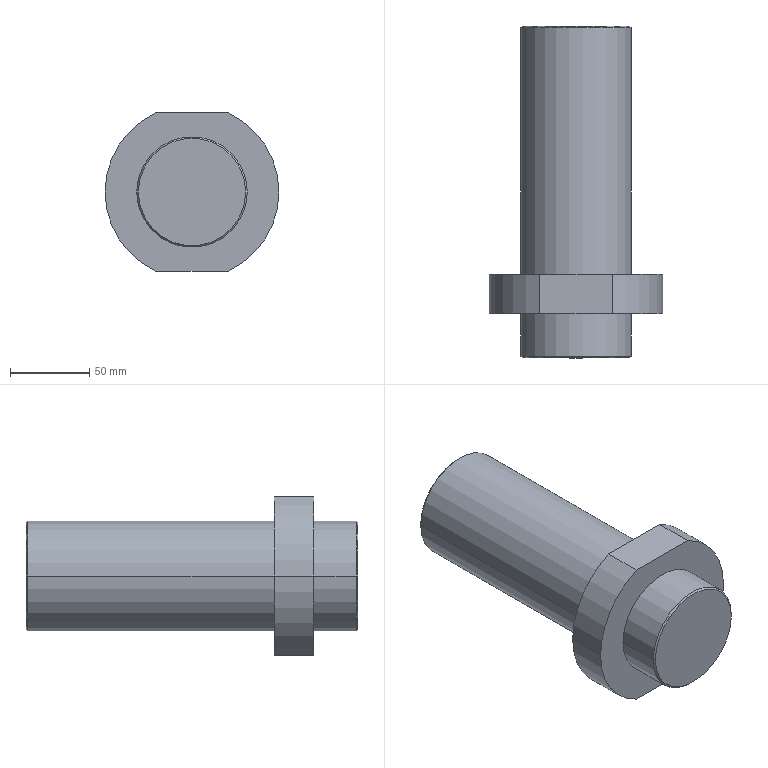Part | SolidWorks | features ICE 1, Revolution 1 | 1 solid | 17 faces | box 110 x 210 x 100 mm | volume 941619 mm3 | cylinder 7 | plane 6 | cone 4 | commonest cylinder face diameters 70 x4 110 x3
STEP:
#1=CARTESIAN_POINT('',(-34.,210.,0.));
#2=VERTEX_POINT('',#1);
#3=CARTESIAN_POINT('',(34.,210.,0.));
#4=VERTEX_POINT('',#3);
#5=CARTESIAN_POINT('',(0.,210.,0.));
#6=DIRECTION('',(0.,1.,0.));
#7=DIRECTION('',(-1.,0.,0.));
#8=AXIS2_PLACEMENT_3D('',#5,#6,#7);
#9=CIRCLE('',#8,34.);
#10=EDGE_CURVE('',#2,#4,#9,.T.);
#11=ORIENTED_EDGE('',*,*,#10,.F.);
#12=CARTESIAN_POINT('',(-35.,209.,0.));
#13=VERTEX_POINT('',#12);
#14=CARTESIAN_POINT('',(-34.,210.,0.));
#15=DIRECTION('',(-0.7071,-0.7071,0.));
#16=VECTOR('',#15,1000.);
#17=LINE('',#14,#16);
#18=EDGE_CURVE('',#2,#13,#17,.T.);
#19=ORIENTED_EDGE('',*,*,#18,.T.);
#20=CARTESIAN_POINT('',(35.,209.,0.));
#21=VERTEX_POINT('',#20);
#22=CARTESIAN_POINT('',(0.,209.,0.));
#23=DIRECTION('',(0.,1.,0.));
#24=DIRECTION('',(-1.,0.,0.));
#25=AXIS2_PLACEMENT_3D('',#22,#23,#24);
#26=CIRCLE('',#25,35.);
#27=EDGE_CURVE('',#13,#21,#26,.T.);
#28=ORIENTED_EDGE('',*,*,#27,.T.);
#29=CARTESIAN_POINT('',(34.,210.,0.));
#30=DIRECTION('',(0.7071,-0.7071,0.));
#31=VECTOR('',#30,1000.);
#32=LINE('',#29,#31);
#33=EDGE_CURVE('',#4,#21,#32,.T.);
#34=ORIENTED_EDGE('',*,*,#33,.F.);
#35=EDGE_LOOP('',(#11,#19,#28,#34));
#36=FACE_OUTER_BOUND('',#35,.T.);
#37=CARTESIAN_POINT('',(0.,210.,0.));
#38=DIRECTION('',(0.,-1.,0.));
#39=DIRECTION('',(1.,0.,0.));
#40=AXIS2_PLACEMENT_3D('',#37,#38,#39);
#41=CONICAL_SURFACE('',#40,34.,0.7854);
#42=ADVANCED_FACE('',(#36),#41,.T.);
#43=CARTESIAN_POINT('',(-35.,53.,0.));
#44=VERTEX_POINT('',#43);
#45=CARTESIAN_POINT('',(35.,53.,0.));
#46=VERTEX_POINT('',#45);
#47=CARTESIAN_POINT('',(0.,53.,0.));
#48=DIRECTION('',(0.,1.,0.));
#49=DIRECTION('',(-1.,0.,0.));
#50=AXIS2_PLACEMENT_3D('',#47,#48,#49);
#51=CIRCLE('',#50,35.);
#52=EDGE_CURVE('',#44,#46,#51,.T.);
#53=ORIENTED_EDGE('',*,*,#52,.T.);
#54=CARTESIAN_POINT('',(35.,210.,0.));
#55=DIRECTION('',(0.,1.,0.));
#56=VECTOR('',#55,1000.);
#57=LINE('',#54,#56);
#58=EDGE_CURVE('',#46,#21,#57,.T.);
#59=ORIENTED_EDGE('',*,*,#58,.T.);
#60=ORIENTED_EDGE('',*,*,#27,.F.);
#61=CARTESIAN_POINT('',(-35.,210.,0.));
#62=DIRECTION('',(0.,1.,0.));
#63=VECTOR('',#62,1000.);
#64=LINE('',#61,#63);
#65=EDGE_CURVE('',#44,#13,#64,.T.);
#66=ORIENTED_EDGE('',*,*,#65,.F.);
#67=EDGE_LOOP('',(#53,#59,#60,#66));
#68=FACE_OUTER_BOUND('',#67,.T.);
#69=CARTESIAN_POINT('',(0.,210.,0.));
#70=DIRECTION('',(0.,1.,0.));
#71=DIRECTION('',(-1.,0.,0.));
#72=AXIS2_PLACEMENT_3D('',#69,#70,#71);
#73=CYLINDRICAL_SURFACE('',#72,35.);
#74=ADVANCED_FACE('',(#68),#73,.T.);
#75=CARTESIAN_POINT('',(-35.,1.,0.));
#76=VERTEX_POINT('',#75);
#77=CARTESIAN_POINT('',(35.,1.,0.));
#78=VERTEX_POINT('',#77);
#79=CARTESIAN_POINT('',(0.,1.,0.));
#80=DIRECTION('',(0.,1.,0.));
#81=DIRECTION('',(-1.,0.,0.));
#82=AXIS2_PLACEMENT_3D('',#79,#80,#81);
#83=CIRCLE('',#82,35.);
#84=EDGE_CURVE('',#76,#78,#83,.T.);
#85=ORIENTED_EDGE('',*,*,#84,.T.);
#86=CARTESIAN_POINT('',(35.,28.,0.));
#87=VERTEX_POINT('',#86);
#88=CARTESIAN_POINT('',(35.,210.,0.));
#89=DIRECTION('',(0.,1.,0.));
#90=VECTOR('',#89,1000.);
#91=LINE('',#88,#90);
#92=EDGE_CURVE('',#78,#87,#91,.T.);
#93=ORIENTED_EDGE('',*,*,#92,.T.);
#94=CARTESIAN_POINT('',(-35.,28.,0.));
#95=VERTEX_POINT('',#94);
#96=CARTESIAN_POINT('',(0.,28.,0.));
#97=DIRECTION('',(0.,1.,0.));
#98=DIRECTION('',(-1.,0.,0.));
#99=AXIS2_PLACEMENT_3D('',#96,#97,#98);
#100=CIRCLE('',#99,35.);
#101=EDGE_CURVE('',#95,#87,#100,.T.);
#102=ORIENTED_EDGE('',*,*,#101,.F.);
#103=CARTESIAN_POINT('',(-35.,210.,0.));
#104=DIRECTION('',(0.,1.,0.));
#105=VECTOR('',#104,1000.);
#106=LINE('',#103,#105);
#107=EDGE_CURVE('',#76,#95,#106,.T.);
#108=ORIENTED_EDGE('',*,*,#107,.F.);
#109=EDGE_LOOP('',(#85,#93,#102,#108));
#110=FACE_OUTER_BOUND('',#109,.T.);
#111=CARTESIAN_POINT('',(0.,210.,0.));
#112=DIRECTION('',(0.,1.,0.));
#113=DIRECTION('',(-1.,0.,0.));
#114=AXIS2_PLACEMENT_3D('',#111,#112,#113);
#115=CYLINDRICAL_SURFACE('',#114,35.);
#116=ADVANCED_FACE('',(#110),#115,.T.);
#117=CARTESIAN_POINT('',(-34.,0.,0.));
#118=VERTEX_POINT('',#117);
#119=CARTESIAN_POINT('',(34.,0.,0.));
#120=VERTEX_POINT('',#119);
#121=CARTESIAN_POINT('',(0.,0.,0.));
#122=DIRECTION('',(0.,1.,0.));
#123=DIRECTION('',(-1.,0.,0.));
#124=AXIS2_PLACEMENT_3D('',#121,#122,#123);
#125=CIRCLE('',#124,34.);
#126=EDGE_CURVE('',#118,#120,#125,.T.);
#127=ORIENTED_EDGE('',*,*,#126,.T.);
#128=CARTESIAN_POINT('',(35.,1.,0.));
#129=DIRECTION('',(0.7071,0.7071,0.));
#130=VECTOR('',#129,1000.);
#131=LINE('',#128,#130);
#132=EDGE_CURVE('',#120,#78,#131,.T.);
#133=ORIENTED_EDGE('',*,*,#132,.T.);
#134=ORIENTED_EDGE('',*,*,#84,.F.);
#135=CARTESIAN_POINT('',(-35.,1.,0.));
#136=DIRECTION('',(-0.7071,0.7071,0.));
#137=VECTOR('',#136,1000.);
#138=LINE('',#135,#137);
#139=EDGE_CURVE('',#118,#76,#138,.T.);
#140=ORIENTED_EDGE('',*,*,#139,.F.);
#141=EDGE_LOOP('',(#127,#133,#134,#140));
#142=FACE_OUTER_BOUND('',#141,.T.);
#143=CARTESIAN_POINT('',(0.,1.,0.));
#144=DIRECTION('',(0.,1.,0.));
#145=DIRECTION('',(-1.,0.,0.));
#146=AXIS2_PLACEMENT_3D('',#143,#144,#145);
#147=CONICAL_SURFACE('',#146,35.,0.7854);
#148=ADVANCED_FACE('',(#142),#147,.T.);
#149=CARTESIAN_POINT('',(-22.913,28.,-50.));
#150=VERTEX_POINT('',#149);
#151=CARTESIAN_POINT('',(-55.,28.,0.));
#152=VERTEX_POINT('',#151);
#153=CARTESIAN_POINT('',(0.,28.,0.));
#154=DIRECTION('',(0.,1.,0.));
#155=DIRECTION('',(-1.,0.,0.));
#156=AXIS2_PLACEMENT_3D('',#153,#154,#155);
#157=CIRCLE('',#156,55.);
#158=EDGE_CURVE('',#150,#152,#157,.T.);
#159=ORIENTED_EDGE('',*,*,#158,.T.);
#160=CARTESIAN_POINT('',(-55.,53.,0.));
#161=VERTEX_POINT('',#160);
#162=CARTESIAN_POINT('',(-55.,210.,0.));
#163=DIRECTION('',(0.,1.,0.));
#164=VECTOR('',#163,1000.);
#165=LINE('',#162,#164);
#166=EDGE_CURVE('',#152,#161,#165,.T.);
#167=ORIENTED_EDGE('',*,*,#166,.T.);
#168=CARTESIAN_POINT('',(-22.913,53.,-50.));
#169=VERTEX_POINT('',#168);
#170=CARTESIAN_POINT('',(0.,53.,0.));
#171=DIRECTION('',(0.,1.,0.));
#172=DIRECTION('',(-1.,0.,0.));
#173=AXIS2_PLACEMENT_3D('',#170,#171,#172);
#174=CIRCLE('',#173,55.);
#175=EDGE_CURVE('',#169,#161,#174,.T.);
#176=ORIENTED_EDGE('',*,*,#175,.F.);
#177=CARTESIAN_POINT('',(-22.913,0.,-50.));
#178=DIRECTION('',(0.,1.,0.));
#179=VECTOR('',#178,1000.);
#180=LINE('',#177,#179);
#181=EDGE_CURVE('',#150,#169,#180,.T.);
#182=ORIENTED_EDGE('',*,*,#181,.F.);
#183=EDGE_LOOP('',(#159,#167,#176,#182));
#184=FACE_OUTER_BOUND('',#183,.T.);
#185=CARTESIAN_POINT('',(0.,210.,0.));
#186=DIRECTION('',(0.,1.,0.));
#187=DIRECTION('',(-1.,0.,0.));
#188=AXIS2_PLACEMENT_3D('',#185,#186,#187);
#189=CYLINDRICAL_SURFACE('',#188,55.);
#190=ADVANCED_FACE('',(#184),#189,.T.);
#191=ORIENTED_EDGE('',*,*,#166,.F.);
#192=CARTESIAN_POINT('',(-22.913,28.,50.));
#193=VERTEX_POINT('',#192);
#194=CARTESIAN_POINT('',(0.,28.,0.));
#195=DIRECTION('',(0.,1.,0.));
#196=DIRECTION('',(-1.,0.,0.));
#197=AXIS2_PLACEMENT_3D('',#194,#195,#196);
#198=CIRCLE('',#197,55.);
#199=EDGE_CURVE('',#152,#193,#198,.T.);
#200=ORIENTED_EDGE('',*,*,#199,.T.);
#201=CARTESIAN_POINT('',(-22.913,53.,50.));
#202=VERTEX_POINT('',#201);
#203=CARTESIAN_POINT('',(-22.913,0.,50.));
#204=DIRECTION('',(0.,1.,0.));
#205=VECTOR('',#204,1000.);
#206=LINE('',#203,#205);
#207=EDGE_CURVE('',#193,#202,#206,.T.);
#208=ORIENTED_EDGE('',*,*,#207,.T.);
#209=CARTESIAN_POINT('',(0.,53.,0.));
#210=DIRECTION('',(0.,1.,0.));
#211=DIRECTION('',(-1.,0.,0.));
#212=AXIS2_PLACEMENT_3D('',#209,#210,#211);
#213=CIRCLE('',#212,55.);
#214=EDGE_CURVE('',#161,#202,#213,.T.);
#215=ORIENTED_EDGE('',*,*,#214,.F.);
#216=EDGE_LOOP('',(#191,#200,#208,#215));
#217=FACE_OUTER_BOUND('',#216,.T.);
#218=CARTESIAN_POINT('',(0.,210.,0.));
#219=DIRECTION('',(0.,1.,0.));
#220=DIRECTION('',(-1.,0.,0.));
#221=AXIS2_PLACEMENT_3D('',#218,#219,#220);
#222=CYLINDRICAL_SURFACE('',#221,55.);
#223=ADVANCED_FACE('',(#217),#222,.T.);
#224=ORIENTED_EDGE('',*,*,#126,.F.);
#225=CARTESIAN_POINT('',(0.,0.,0.));
#226=DIRECTION('',(0.,1.,0.));
#227=DIRECTION('',(-1.,0.,0.));
#228=AXIS2_PLACEMENT_3D('',#225,#226,#227);
#229=CIRCLE('',#228,34.);
#230=EDGE_CURVE('',#120,#118,#229,.T.);
#231=ORIENTED_EDGE('',*,*,#230,.F.);
#232=EDGE_LOOP('',(#224,#231));
#233=FACE_OUTER_BOUND('',#232,.T.);
#234=CARTESIAN_POINT('',(0.,0.,0.));
#235=DIRECTION('',(0.,-1.,0.));
#236=DIRECTION('',(1.,0.,0.));
#237=AXIS2_PLACEMENT_3D('',#234,#235,#236);
#238=PLANE('',#237);
#239=ADVANCED_FACE('',(#233),#238,.T.);
#240=ORIENTED_EDGE('',*,*,#132,.F.);
#241=ORIENTED_EDGE('',*,*,#230,.T.);
#242=ORIENTED_EDGE('',*,*,#139,.T.);
#243=CARTESIAN_POINT('',(0.,1.,0.));
#244=DIRECTION('',(0.,1.,0.));
#245=DIRECTION('',(-1.,0.,0.));
#246=AXIS2_PLACEMENT_3D('',#243,#244,#245);
#247=CIRCLE('',#246,35.);
#248=EDGE_CURVE('',#78,#76,#247,.T.);
#249=ORIENTED_EDGE('',*,*,#248,.F.);
#250=EDGE_LOOP('',(#240,#241,#242,#249));
#251=FACE_OUTER_BOUND('',#250,.T.);
#252=CARTESIAN_POINT('',(0.,1.,0.));
#253=DIRECTION('',(0.,1.,0.));
#254=DIRECTION('',(-1.,0.,0.));
#255=AXIS2_PLACEMENT_3D('',#252,#253,#254);
#256=CONICAL_SURFACE('',#255,35.,0.7854);
#257=ADVANCED_FACE('',(#251),#256,.T.);
#258=ORIENTED_EDGE('',*,*,#92,.F.);
#259=ORIENTED_EDGE('',*,*,#248,.T.);
#260=ORIENTED_EDGE('',*,*,#107,.T.);
#261=CARTESIAN_POINT('',(0.,28.,0.));
#262=DIRECTION('',(0.,1.,0.));
#263=DIRECTION('',(-1.,0.,0.));
#264=AXIS2_PLACEMENT_3D('',#261,#262,#263);
#265=CIRCLE('',#264,35.);
#266=EDGE_CURVE('',#87,#95,#265,.T.);
#267=ORIENTED_EDGE('',*,*,#266,.F.);
#268=EDGE_LOOP('',(#258,#259,#260,#267));
#269=FACE_OUTER_BOUND('',#268,.T.);
#270=CARTESIAN_POINT('',(0.,210.,0.));
#271=DIRECTION('',(0.,1.,0.));
#272=DIRECTION('',(-1.,0.,0.));
#273=AXIS2_PLACEMENT_3D('',#270,#271,#272);
#274=CYLINDRICAL_SURFACE('',#273,35.);
#275=ADVANCED_FACE('',(#269),#274,.T.);
#276=CARTESIAN_POINT('',(22.913,28.,50.));
#277=VERTEX_POINT('',#276);
#278=CARTESIAN_POINT('',(-35.,28.,50.));
#279=DIRECTION('',(1.,0.,0.));
#280=VECTOR('',#279,1000.);
#281=LINE('',#278,#280);
#282=EDGE_CURVE('',#193,#277,#281,.T.);
#283=ORIENTED_EDGE('',*,*,#282,.F.);
#284=ORIENTED_EDGE('',*,*,#199,.F.);
#285=ORIENTED_EDGE('',*,*,#158,.F.);
#286=CARTESIAN_POINT('',(22.913,28.,-50.));
#287=VERTEX_POINT('',#286);
#288=CARTESIAN_POINT('',(-35.,28.,-50.));
#289=DIRECTION('',(-1.,0.,0.));
#290=VECTOR('',#289,1000.);
#291=LINE('',#288,#290);
#292=EDGE_CURVE('',#287,#150,#291,.T.);
#293=ORIENTED_EDGE('',*,*,#292,.F.);
#294=CARTESIAN_POINT('',(0.,28.,0.));
#295=DIRECTION('',(0.,1.,0.));
#296=DIRECTION('',(-1.,0.,0.));
#297=AXIS2_PLACEMENT_3D('',#294,#295,#296);
#298=CIRCLE('',#297,55.);
#299=EDGE_CURVE('',#277,#287,#298,.T.);
#300=ORIENTED_EDGE('',*,*,#299,.F.);
#301=EDGE_LOOP('',(#283,#284,#285,#293,#300));
#302=FACE_OUTER_BOUND('',#301,.T.);
#303=ORIENTED_EDGE('',*,*,#101,.T.);
#304=ORIENTED_EDGE('',*,*,#266,.T.);
#305=EDGE_LOOP('',(#303,#304));
#306=FACE_BOUND('',#305,.T.);
#307=CARTESIAN_POINT('',(-35.,28.,0.));
#308=DIRECTION('',(0.,-1.,0.));
#309=DIRECTION('',(1.,0.,0.));
#310=AXIS2_PLACEMENT_3D('',#307,#308,#309);
#311=PLANE('',#310);
#312=ADVANCED_FACE('',(#302,#306),#311,.T.);
#313=CARTESIAN_POINT('',(22.913,53.,50.));
#314=VERTEX_POINT('',#313);
#315=CARTESIAN_POINT('',(22.913,0.,50.));
#316=DIRECTION('',(0.,1.,0.));
#317=VECTOR('',#316,1000.);
#318=LINE('',#315,#317);
#319=EDGE_CURVE('',#277,#314,#318,.T.);
#320=ORIENTED_EDGE('',*,*,#319,.F.);
#321=ORIENTED_EDGE('',*,*,#299,.T.);
#322=CARTESIAN_POINT('',(22.913,53.,-50.));
#323=VERTEX_POINT('',#322);
#324=CARTESIAN_POINT('',(22.913,0.,-50.));
#325=DIRECTION('',(0.,1.,0.));
#326=VECTOR('',#325,1000.);
#327=LINE('',#324,#326);
#328=EDGE_CURVE('',#287,#323,#327,.T.);
#329=ORIENTED_EDGE('',*,*,#328,.T.);
#330=CARTESIAN_POINT('',(0.,53.,0.));
#331=DIRECTION('',(0.,1.,0.));
#332=DIRECTION('',(-1.,0.,0.));
#333=AXIS2_PLACEMENT_3D('',#330,#331,#332);
#334=CIRCLE('',#333,55.);
#335=EDGE_CURVE('',#314,#323,#334,.T.);
#336=ORIENTED_EDGE('',*,*,#335,.F.);
#337=EDGE_LOOP('',(#320,#321,#329,#336));
#338=FACE_OUTER_BOUND('',#337,.T.);
#339=CARTESIAN_POINT('',(0.,210.,0.));
#340=DIRECTION('',(0.,1.,0.));
#341=DIRECTION('',(-1.,0.,0.));
#342=AXIS2_PLACEMENT_3D('',#339,#340,#341);
#343=CYLINDRICAL_SURFACE('',#342,55.);
#344=ADVANCED_FACE('',(#338),#343,.T.);
#345=CARTESIAN_POINT('',(-22.913,53.,50.));
#346=DIRECTION('',(-1.,0.,0.));
#347=VECTOR('',#346,1000.);
#348=LINE('',#345,#347);
#349=EDGE_CURVE('',#314,#202,#348,.T.);
#350=ORIENTED_EDGE('',*,*,#349,.F.);
#351=ORIENTED_EDGE('',*,*,#335,.T.);
#352=CARTESIAN_POINT('',(-22.913,53.,-50.));
#353=DIRECTION('',(1.,0.,0.));
#354=VECTOR('',#353,1000.);
#355=LINE('',#352,#354);
#356=EDGE_CURVE('',#169,#323,#355,.T.);
#357=ORIENTED_EDGE('',*,*,#356,.F.);
#358=ORIENTED_EDGE('',*,*,#175,.T.);
#359=ORIENTED_EDGE('',*,*,#214,.T.);
#360=EDGE_LOOP('',(#350,#351,#357,#358,#359));
#361=FACE_OUTER_BOUND('',#360,.T.);
#362=ORIENTED_EDGE('',*,*,#52,.F.);
#363=CARTESIAN_POINT('',(0.,53.,0.));
#364=DIRECTION('',(0.,1.,0.));
#365=DIRECTION('',(-1.,0.,0.));
#366=AXIS2_PLACEMENT_3D('',#363,#364,#365);
#367=CIRCLE('',#366,35.);
#368=EDGE_CURVE('',#46,#44,#367,.T.);
#369=ORIENTED_EDGE('',*,*,#368,.F.);
#370=EDGE_LOOP('',(#362,#369));
#371=FACE_BOUND('',#370,.T.);
#372=CARTESIAN_POINT('',(-55.,53.,0.));
#373=DIRECTION('',(0.,1.,0.));
#374=DIRECTION('',(-1.,0.,0.));
#375=AXIS2_PLACEMENT_3D('',#372,#373,#374);
#376=PLANE('',#375);
#377=ADVANCED_FACE('',(#361,#371),#376,.T.);
#378=ORIENTED_EDGE('',*,*,#58,.F.);
#379=ORIENTED_EDGE('',*,*,#368,.T.);
#380=ORIENTED_EDGE('',*,*,#65,.T.);
#381=CARTESIAN_POINT('',(0.,209.,0.));
#382=DIRECTION('',(0.,1.,0.));
#383=DIRECTION('',(-1.,0.,0.));
#384=AXIS2_PLACEMENT_3D('',#381,#382,#383);
#385=CIRCLE('',#384,35.);
#386=EDGE_CURVE('',#21,#13,#385,.T.);
#387=ORIENTED_EDGE('',*,*,#386,.F.);
#388=EDGE_LOOP('',(#378,#379,#380,#387));
#389=FACE_OUTER_BOUND('',#388,.T.);
#390=CARTESIAN_POINT('',(0.,210.,0.));
#391=DIRECTION('',(0.,1.,0.));
#392=DIRECTION('',(-1.,0.,0.));
#393=AXIS2_PLACEMENT_3D('',#390,#391,#392);
#394=CYLINDRICAL_SURFACE('',#393,35.);
#395=ADVANCED_FACE('',(#389),#394,.T.);
#396=ORIENTED_EDGE('',*,*,#18,.F.);
#397=CARTESIAN_POINT('',(0.,210.,0.));
#398=DIRECTION('',(0.,1.,0.));
#399=DIRECTION('',(-1.,0.,0.));
#400=AXIS2_PLACEMENT_3D('',#397,#398,#399);
#401=CIRCLE('',#400,34.);
#402=EDGE_CURVE('',#4,#2,#401,.T.);
#403=ORIENTED_EDGE('',*,*,#402,.F.);
#404=ORIENTED_EDGE('',*,*,#33,.T.);
#405=ORIENTED_EDGE('',*,*,#386,.T.);
#406=EDGE_LOOP('',(#396,#403,#404,#405));
#407=FACE_OUTER_BOUND('',#406,.T.);
#408=CARTESIAN_POINT('',(0.,210.,0.));
#409=DIRECTION('',(0.,-1.,0.));
#410=DIRECTION('',(1.,0.,0.));
#411=AXIS2_PLACEMENT_3D('',#408,#409,#410);
#412=CONICAL_SURFACE('',#411,34.,0.7854);
#413=ADVANCED_FACE('',(#407),#412,.T.);
#414=ORIENTED_EDGE('',*,*,#402,.T.);
#415=ORIENTED_EDGE('',*,*,#10,.T.);
#416=EDGE_LOOP('',(#414,#415));
#417=FACE_OUTER_BOUND('',#416,.T.);
#418=CARTESIAN_POINT('',(-34.,210.,0.));
#419=DIRECTION('',(0.,1.,0.));
#420=DIRECTION('',(-1.,0.,0.));
#421=AXIS2_PLACEMENT_3D('',#418,#419,#420);
#422=PLANE('',#421);
#423=ADVANCED_FACE('',(#417),#422,.T.);
#424=ORIENTED_EDGE('',*,*,#292,.T.);
#425=ORIENTED_EDGE('',*,*,#181,.T.);
#426=ORIENTED_EDGE('',*,*,#356,.T.);
#427=ORIENTED_EDGE('',*,*,#328,.F.);
#428=EDGE_LOOP('',(#424,#425,#426,#427));
#429=FACE_OUTER_BOUND('',#428,.T.);
#430=CARTESIAN_POINT('',(-22.913,0.,-50.));
#431=DIRECTION('',(0.,0.,1.));
#432=DIRECTION('',(1.,0.,0.));
#433=AXIS2_PLACEMENT_3D('',#430,#431,#432);
#434=PLANE('',#433);
#435=ADVANCED_FACE('',(#429),#434,.F.);
#436=ORIENTED_EDGE('',*,*,#282,.T.);
#437=ORIENTED_EDGE('',*,*,#319,.T.);
#438=ORIENTED_EDGE('',*,*,#349,.T.);
#439=ORIENTED_EDGE('',*,*,#207,.F.);
#440=EDGE_LOOP('',(#436,#437,#438,#439));
#441=FACE_OUTER_BOUND('',#440,.T.);
#442=CARTESIAN_POINT('',(-22.913,0.,50.));
#443=DIRECTION('',(0.,0.,-1.));
#444=DIRECTION('',(-1.,0.,0.));
#445=AXIS2_PLACEMENT_3D('',#442,#443,#444);
#446=PLANE('',#445);
#447=ADVANCED_FACE('',(#441),#446,.F.);
#448=CLOSED_SHELL('',(#42,#74,#116,#148,#190,#223,#239,#257,#275,#312,#344,#377,#395,#413,#423,#435,#447));
#449=MANIFOLD_SOLID_BREP('',#448);
#450=CARTESIAN_POINT('',(0.,0.,0.));
#451=DIRECTION('',(0.,0.,1.));
#452=DIRECTION('',(1.,0.,0.));
#453=AXIS2_PLACEMENT_3D('',#450,#451,#452);
#454=(LENGTH_UNIT()NAMED_UNIT(*)SI_UNIT(.MILLI.,.METRE.));
#455=UNCERTAINTY_MEASURE_WITH_UNIT(LENGTH_MEASURE(0.00001),#454,'','');
#456=(NAMED_UNIT(*)PLANE_ANGLE_UNIT()SI_UNIT($,.RADIAN.));
#457=(NAMED_UNIT(*)SI_UNIT($,.STERADIAN.)SOLID_ANGLE_UNIT());
#458=(GEOMETRIC_REPRESENTATION_CONTEXT(3)GLOBAL_UNCERTAINTY_ASSIGNED_CONTEXT((#455))GLOBAL_UNIT_ASSIGNED_CONTEXT((#454,#456,#457))REPRESENTATION_CONTEXT('',''));
#459=ADVANCED_BREP_SHAPE_REPRESENTATION('',(#449,#453),#458);